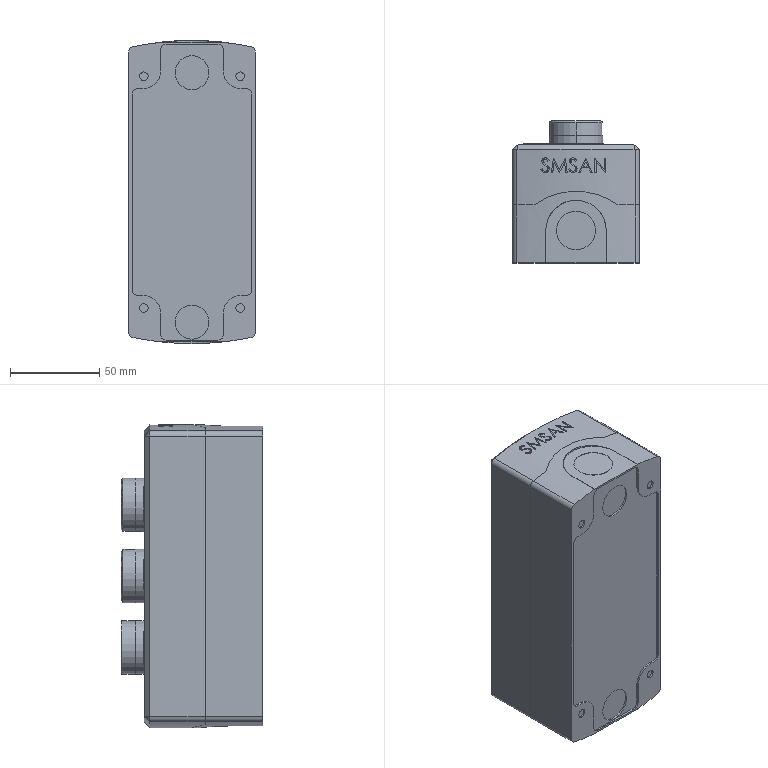Part | STEP file | 11M | 2 solids | 537 faces | box 71 x 79.5 x 170.1 mm | volume 187590 mm3 | plane 282 | cylinder 122 | spline 119 | cone 14 | commonest cylinder face diameters 6 x16 2 x12 26.5 x10 4.8 x8 8 x8 9 x8